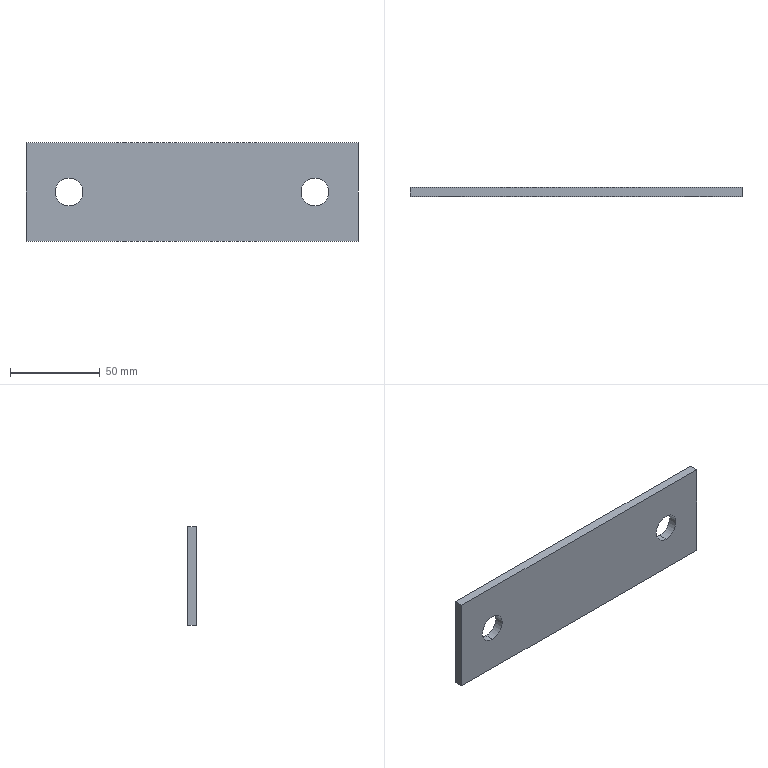Part | STEP file | Produce dryer bearing housing pad plate | 1 solid | 10 faces | box 185 x 5 x 55 mm | volume 48988 mm3 | plane 6 | cylinder 4 | commonest cylinder face diameters 15.5 x4
STEP:
#1=CARTESIAN_POINT('',(24.,0.,-7.75));
#2=VERTEX_POINT('',#1);
#3=CARTESIAN_POINT('',(24.,0.,7.75));
#4=VERTEX_POINT('',#3);
#5=CARTESIAN_POINT('',(24.,0.,0.));
#6=DIRECTION('',(0.,1.,0.));
#7=DIRECTION('',(0.,0.,1.));
#8=AXIS2_PLACEMENT_3D('',#5,#6,#7);
#9=CIRCLE('',#8,7.75);
#10=EDGE_CURVE('',#2,#4,#9,.T.);
#11=ORIENTED_EDGE('',*,*,#10,.F.);
#12=CARTESIAN_POINT('',(24.,5.,-7.75));
#13=VERTEX_POINT('',#12);
#14=CARTESIAN_POINT('',(24.,5.,-7.75));
#15=DIRECTION('',(0.,1.,0.));
#16=VECTOR('',#15,1000.);
#17=LINE('',#14,#16);
#18=EDGE_CURVE('',#2,#13,#17,.T.);
#19=ORIENTED_EDGE('',*,*,#18,.T.);
#20=CARTESIAN_POINT('',(24.,5.,7.75));
#21=VERTEX_POINT('',#20);
#22=CARTESIAN_POINT('',(24.,5.,0.));
#23=DIRECTION('',(0.,1.,0.));
#24=DIRECTION('',(0.,0.,1.));
#25=AXIS2_PLACEMENT_3D('',#22,#23,#24);
#26=CIRCLE('',#25,7.75);
#27=EDGE_CURVE('',#13,#21,#26,.T.);
#28=ORIENTED_EDGE('',*,*,#27,.T.);
#29=CARTESIAN_POINT('',(24.,5.,7.75));
#30=DIRECTION('',(0.,1.,0.));
#31=VECTOR('',#30,1000.);
#32=LINE('',#29,#31);
#33=EDGE_CURVE('',#4,#21,#32,.T.);
#34=ORIENTED_EDGE('',*,*,#33,.F.);
#35=EDGE_LOOP('',(#11,#19,#28,#34));
#36=FACE_OUTER_BOUND('',#35,.T.);
#37=CARTESIAN_POINT('',(24.,5.,0.));
#38=DIRECTION('',(0.,1.,0.));
#39=DIRECTION('',(0.,0.,1.));
#40=AXIS2_PLACEMENT_3D('',#37,#38,#39);
#41=CYLINDRICAL_SURFACE('',#40,7.75);
#42=ADVANCED_FACE('',(#36),#41,.F.);
#43=CARTESIAN_POINT('',(161.,0.,-7.75));
#44=VERTEX_POINT('',#43);
#45=CARTESIAN_POINT('',(161.,0.,7.75));
#46=VERTEX_POINT('',#45);
#47=CARTESIAN_POINT('',(161.,0.,0.));
#48=DIRECTION('',(0.,1.,0.));
#49=DIRECTION('',(0.,0.,1.));
#50=AXIS2_PLACEMENT_3D('',#47,#48,#49);
#51=CIRCLE('',#50,7.75);
#52=EDGE_CURVE('',#44,#46,#51,.T.);
#53=ORIENTED_EDGE('',*,*,#52,.F.);
#54=CARTESIAN_POINT('',(161.,5.,-7.75));
#55=VERTEX_POINT('',#54);
#56=CARTESIAN_POINT('',(161.,5.,-7.75));
#57=DIRECTION('',(0.,1.,0.));
#58=VECTOR('',#57,1000.);
#59=LINE('',#56,#58);
#60=EDGE_CURVE('',#44,#55,#59,.T.);
#61=ORIENTED_EDGE('',*,*,#60,.T.);
#62=CARTESIAN_POINT('',(161.,5.,7.75));
#63=VERTEX_POINT('',#62);
#64=CARTESIAN_POINT('',(161.,5.,0.));
#65=DIRECTION('',(0.,1.,0.));
#66=DIRECTION('',(0.,0.,1.));
#67=AXIS2_PLACEMENT_3D('',#64,#65,#66);
#68=CIRCLE('',#67,7.75);
#69=EDGE_CURVE('',#55,#63,#68,.T.);
#70=ORIENTED_EDGE('',*,*,#69,.T.);
#71=CARTESIAN_POINT('',(161.,5.,7.75));
#72=DIRECTION('',(0.,1.,0.));
#73=VECTOR('',#72,1000.);
#74=LINE('',#71,#73);
#75=EDGE_CURVE('',#46,#63,#74,.T.);
#76=ORIENTED_EDGE('',*,*,#75,.F.);
#77=EDGE_LOOP('',(#53,#61,#70,#76));
#78=FACE_OUTER_BOUND('',#77,.T.);
#79=CARTESIAN_POINT('',(161.,5.,0.));
#80=DIRECTION('',(0.,1.,0.));
#81=DIRECTION('',(0.,0.,1.));
#82=AXIS2_PLACEMENT_3D('',#79,#80,#81);
#83=CYLINDRICAL_SURFACE('',#82,7.75);
#84=ADVANCED_FACE('',(#78),#83,.F.);
#85=CARTESIAN_POINT('',(185.,0.,27.5));
#86=VERTEX_POINT('',#85);
#87=CARTESIAN_POINT('',(185.,5.,27.5));
#88=VERTEX_POINT('',#87);
#89=CARTESIAN_POINT('',(185.,0.,27.5));
#90=DIRECTION('',(0.,1.,0.));
#91=VECTOR('',#90,1000.);
#92=LINE('',#89,#91);
#93=EDGE_CURVE('',#86,#88,#92,.T.);
#94=ORIENTED_EDGE('',*,*,#93,.T.);
#95=CARTESIAN_POINT('',(0.,5.,27.5));
#96=VERTEX_POINT('',#95);
#97=CARTESIAN_POINT('',(0.,5.,27.5));
#98=DIRECTION('',(1.,0.,0.));
#99=VECTOR('',#98,1000.);
#100=LINE('',#97,#99);
#101=EDGE_CURVE('',#96,#88,#100,.T.);
#102=ORIENTED_EDGE('',*,*,#101,.F.);
#103=CARTESIAN_POINT('',(0.,0.,27.5));
#104=VERTEX_POINT('',#103);
#105=CARTESIAN_POINT('',(0.,0.,27.5));
#106=DIRECTION('',(0.,1.,0.));
#107=VECTOR('',#106,1000.);
#108=LINE('',#105,#107);
#109=EDGE_CURVE('',#104,#96,#108,.T.);
#110=ORIENTED_EDGE('',*,*,#109,.F.);
#111=CARTESIAN_POINT('',(0.,0.,27.5));
#112=DIRECTION('',(1.,0.,0.));
#113=VECTOR('',#112,1000.);
#114=LINE('',#111,#113);
#115=EDGE_CURVE('',#104,#86,#114,.T.);
#116=ORIENTED_EDGE('',*,*,#115,.T.);
#117=EDGE_LOOP('',(#94,#102,#110,#116));
#118=FACE_OUTER_BOUND('',#117,.T.);
#119=CARTESIAN_POINT('',(195.,5.737,27.5));
#120=DIRECTION('',(0.,0.,1.));
#121=DIRECTION('',(1.,0.,0.));
#122=AXIS2_PLACEMENT_3D('',#119,#120,#121);
#123=PLANE('',#122);
#124=ADVANCED_FACE('',(#118),#123,.T.);
#125=CARTESIAN_POINT('',(185.,5.,-27.5));
#126=VERTEX_POINT('',#125);
#127=CARTESIAN_POINT('',(185.,5.,27.5));
#128=DIRECTION('',(0.,0.,1.));
#129=VECTOR('',#128,1000.);
#130=LINE('',#127,#129);
#131=EDGE_CURVE('',#126,#88,#130,.T.);
#132=ORIENTED_EDGE('',*,*,#131,.F.);
#133=CARTESIAN_POINT('',(0.,5.,-27.5));
#134=VERTEX_POINT('',#133);
#135=CARTESIAN_POINT('',(0.,5.,-27.5));
#136=DIRECTION('',(1.,0.,0.));
#137=VECTOR('',#136,1000.);
#138=LINE('',#135,#137);
#139=EDGE_CURVE('',#134,#126,#138,.T.);
#140=ORIENTED_EDGE('',*,*,#139,.F.);
#141=CARTESIAN_POINT('',(0.,5.,27.5));
#142=DIRECTION('',(0.,0.,-1.));
#143=VECTOR('',#142,1000.);
#144=LINE('',#141,#143);
#145=EDGE_CURVE('',#96,#134,#144,.T.);
#146=ORIENTED_EDGE('',*,*,#145,.F.);
#147=ORIENTED_EDGE('',*,*,#101,.T.);
#148=EDGE_LOOP('',(#132,#140,#146,#147));
#149=FACE_OUTER_BOUND('',#148,.T.);
#150=CARTESIAN_POINT('',(24.,5.,0.));
#151=DIRECTION('',(0.,1.,0.));
#152=DIRECTION('',(0.,0.,1.));
#153=AXIS2_PLACEMENT_3D('',#150,#151,#152);
#154=CIRCLE('',#153,7.75);
#155=EDGE_CURVE('',#21,#13,#154,.T.);
#156=ORIENTED_EDGE('',*,*,#155,.F.);
#157=ORIENTED_EDGE('',*,*,#27,.F.);
#158=EDGE_LOOP('',(#156,#157));
#159=FACE_BOUND('',#158,.T.);
#160=CARTESIAN_POINT('',(161.,5.,0.));
#161=DIRECTION('',(0.,1.,0.));
#162=DIRECTION('',(0.,0.,1.));
#163=AXIS2_PLACEMENT_3D('',#160,#161,#162);
#164=CIRCLE('',#163,7.75);
#165=EDGE_CURVE('',#63,#55,#164,.T.);
#166=ORIENTED_EDGE('',*,*,#165,.F.);
#167=ORIENTED_EDGE('',*,*,#69,.F.);
#168=EDGE_LOOP('',(#166,#167));
#169=FACE_BOUND('',#168,.T.);
#170=CARTESIAN_POINT('',(0.,5.,27.5));
#171=DIRECTION('',(0.,1.,0.));
#172=DIRECTION('',(0.,0.,1.));
#173=AXIS2_PLACEMENT_3D('',#170,#171,#172);
#174=PLANE('',#173);
#175=ADVANCED_FACE('',(#149,#159,#169),#174,.T.);
#176=CARTESIAN_POINT('',(0.,0.,-27.5));
#177=VERTEX_POINT('',#176);
#178=CARTESIAN_POINT('',(0.,0.,-27.5));
#179=DIRECTION('',(0.,1.,0.));
#180=VECTOR('',#179,1000.);
#181=LINE('',#178,#180);
#182=EDGE_CURVE('',#177,#134,#181,.T.);
#183=ORIENTED_EDGE('',*,*,#182,.F.);
#184=CARTESIAN_POINT('',(0.,0.,27.5));
#185=DIRECTION('',(0.,0.,-1.));
#186=VECTOR('',#185,1000.);
#187=LINE('',#184,#186);
#188=EDGE_CURVE('',#104,#177,#187,.T.);
#189=ORIENTED_EDGE('',*,*,#188,.F.);
#190=ORIENTED_EDGE('',*,*,#109,.T.);
#191=ORIENTED_EDGE('',*,*,#145,.T.);
#192=EDGE_LOOP('',(#183,#189,#190,#191));
#193=FACE_OUTER_BOUND('',#192,.T.);
#194=CARTESIAN_POINT('',(0.,0.,27.5));
#195=DIRECTION('',(-1.,0.,0.));
#196=DIRECTION('',(0.,0.,1.));
#197=AXIS2_PLACEMENT_3D('',#194,#195,#196);
#198=PLANE('',#197);
#199=ADVANCED_FACE('',(#193),#198,.T.);
#200=CARTESIAN_POINT('',(24.,0.,0.));
#201=DIRECTION('',(0.,1.,0.));
#202=DIRECTION('',(0.,0.,1.));
#203=AXIS2_PLACEMENT_3D('',#200,#201,#202);
#204=CIRCLE('',#203,7.75);
#205=EDGE_CURVE('',#4,#2,#204,.T.);
#206=ORIENTED_EDGE('',*,*,#205,.T.);
#207=ORIENTED_EDGE('',*,*,#10,.T.);
#208=EDGE_LOOP('',(#206,#207));
#209=FACE_BOUND('',#208,.T.);
#210=CARTESIAN_POINT('',(161.,0.,0.));
#211=DIRECTION('',(0.,1.,0.));
#212=DIRECTION('',(0.,0.,1.));
#213=AXIS2_PLACEMENT_3D('',#210,#211,#212);
#214=CIRCLE('',#213,7.75);
#215=EDGE_CURVE('',#46,#44,#214,.T.);
#216=ORIENTED_EDGE('',*,*,#215,.T.);
#217=ORIENTED_EDGE('',*,*,#52,.T.);
#218=EDGE_LOOP('',(#216,#217));
#219=FACE_BOUND('',#218,.T.);
#220=CARTESIAN_POINT('',(185.,0.,-27.5));
#221=VERTEX_POINT('',#220);
#222=CARTESIAN_POINT('',(0.,0.,-27.5));
#223=DIRECTION('',(1.,0.,0.));
#224=VECTOR('',#223,1000.);
#225=LINE('',#222,#224);
#226=EDGE_CURVE('',#177,#221,#225,.T.);
#227=ORIENTED_EDGE('',*,*,#226,.T.);
#228=CARTESIAN_POINT('',(185.,0.,-27.5));
#229=DIRECTION('',(0.,0.,1.));
#230=VECTOR('',#229,1000.);
#231=LINE('',#228,#230);
#232=EDGE_CURVE('',#221,#86,#231,.T.);
#233=ORIENTED_EDGE('',*,*,#232,.T.);
#234=ORIENTED_EDGE('',*,*,#115,.F.);
#235=ORIENTED_EDGE('',*,*,#188,.T.);
#236=EDGE_LOOP('',(#227,#233,#234,#235));
#237=FACE_OUTER_BOUND('',#236,.T.);
#238=CARTESIAN_POINT('',(0.,0.,27.5));
#239=DIRECTION('',(0.,1.,0.));
#240=DIRECTION('',(0.,0.,1.));
#241=AXIS2_PLACEMENT_3D('',#238,#239,#240);
#242=PLANE('',#241);
#243=ADVANCED_FACE('',(#209,#219,#237),#242,.F.);
#244=ORIENTED_EDGE('',*,*,#139,.T.);
#245=CARTESIAN_POINT('',(185.,0.,-27.5));
#246=DIRECTION('',(0.,1.,0.));
#247=VECTOR('',#246,1000.);
#248=LINE('',#245,#247);
#249=EDGE_CURVE('',#221,#126,#248,.T.);
#250=ORIENTED_EDGE('',*,*,#249,.F.);
#251=ORIENTED_EDGE('',*,*,#226,.F.);
#252=ORIENTED_EDGE('',*,*,#182,.T.);
#253=EDGE_LOOP('',(#244,#250,#251,#252));
#254=FACE_OUTER_BOUND('',#253,.T.);
#255=CARTESIAN_POINT('',(194.263,5.737,-27.5));
#256=DIRECTION('',(0.,0.,1.));
#257=DIRECTION('',(1.,0.,0.));
#258=AXIS2_PLACEMENT_3D('',#255,#256,#257);
#259=PLANE('',#258);
#260=ADVANCED_FACE('',(#254),#259,.F.);
#261=ORIENTED_EDGE('',*,*,#60,.F.);
#262=ORIENTED_EDGE('',*,*,#215,.F.);
#263=ORIENTED_EDGE('',*,*,#75,.T.);
#264=ORIENTED_EDGE('',*,*,#165,.T.);
#265=EDGE_LOOP('',(#261,#262,#263,#264));
#266=FACE_OUTER_BOUND('',#265,.T.);
#267=CARTESIAN_POINT('',(161.,5.,0.));
#268=DIRECTION('',(0.,1.,0.));
#269=DIRECTION('',(0.,0.,1.));
#270=AXIS2_PLACEMENT_3D('',#267,#268,#269);
#271=CYLINDRICAL_SURFACE('',#270,7.75);
#272=ADVANCED_FACE('',(#266),#271,.F.);
#273=ORIENTED_EDGE('',*,*,#18,.F.);
#274=ORIENTED_EDGE('',*,*,#205,.F.);
#275=ORIENTED_EDGE('',*,*,#33,.T.);
#276=ORIENTED_EDGE('',*,*,#155,.T.);
#277=EDGE_LOOP('',(#273,#274,#275,#276));
#278=FACE_OUTER_BOUND('',#277,.T.);
#279=CARTESIAN_POINT('',(24.,5.,0.));
#280=DIRECTION('',(0.,1.,0.));
#281=DIRECTION('',(0.,0.,1.));
#282=AXIS2_PLACEMENT_3D('',#279,#280,#281);
#283=CYLINDRICAL_SURFACE('',#282,7.75);
#284=ADVANCED_FACE('',(#278),#283,.F.);
#285=ORIENTED_EDGE('',*,*,#131,.T.);
#286=ORIENTED_EDGE('',*,*,#93,.F.);
#287=ORIENTED_EDGE('',*,*,#232,.F.);
#288=ORIENTED_EDGE('',*,*,#249,.T.);
#289=EDGE_LOOP('',(#285,#286,#287,#288));
#290=FACE_OUTER_BOUND('',#289,.T.);
#291=CARTESIAN_POINT('',(185.,0.,-27.5));
#292=DIRECTION('',(-1.,0.,0.));
#293=DIRECTION('',(0.,0.,1.));
#294=AXIS2_PLACEMENT_3D('',#291,#292,#293);
#295=PLANE('',#294);
#296=ADVANCED_FACE('',(#290),#295,.F.);
#297=CLOSED_SHELL('',(#42,#84,#124,#175,#199,#243,#260,#272,#284,#296));
#298=MANIFOLD_SOLID_BREP('',#297);
#299=CARTESIAN_POINT('',(0.,0.,0.));
#300=DIRECTION('',(0.,0.,1.));
#301=DIRECTION('',(1.,0.,0.));
#302=AXIS2_PLACEMENT_3D('',#299,#300,#301);
#303=(LENGTH_UNIT()NAMED_UNIT(*)SI_UNIT(.MILLI.,.METRE.));
#304=UNCERTAINTY_MEASURE_WITH_UNIT(LENGTH_MEASURE(0.00001),#303,'','');
#305=(NAMED_UNIT(*)PLANE_ANGLE_UNIT()SI_UNIT($,.RADIAN.));
#306=(NAMED_UNIT(*)SI_UNIT($,.STERADIAN.)SOLID_ANGLE_UNIT());
#307=(GEOMETRIC_REPRESENTATION_CONTEXT(3)GLOBAL_UNCERTAINTY_ASSIGNED_CONTEXT((#304))GLOBAL_UNIT_ASSIGNED_CONTEXT((#303,#305,#306))REPRESENTATION_CONTEXT('',''));
#308=ADVANCED_BREP_SHAPE_REPRESENTATION('',(#298,#302),#307);